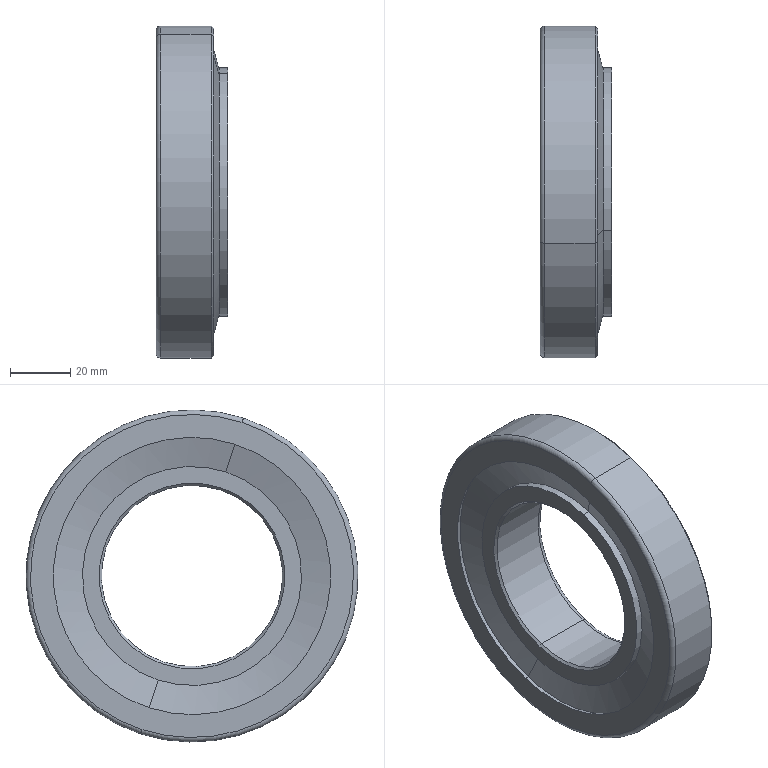Part | STEP file | Input 18 | 1 solid | 35 faces | box 23.75 x 110 x 110 mm | volume 129421 mm3 | cone 18 | cylinder 8 | plane 5 | torus 4 | commonest cylinder face diameters 60 x2 72.536 x2 82.548 x2 110 x2